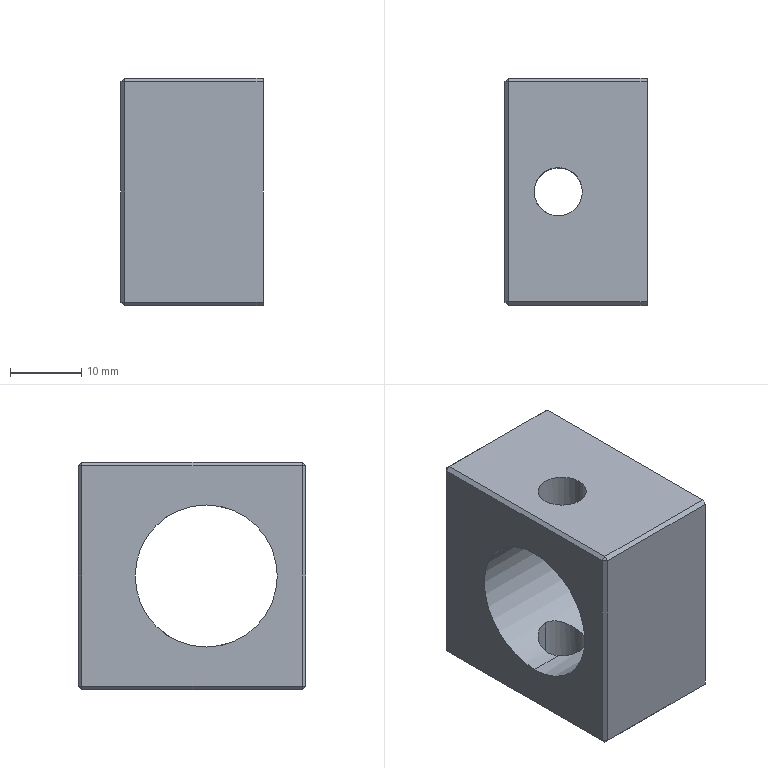Part | STEP file | 02-13 Tensioning block 2 | 1 solid | 27 faces | box 20 x 32 x 32 mm | volume 13018 mm3 | plane 19 | cylinder 8 | commonest cylinder face diameters 6.8 x4 20 x2 24 x2